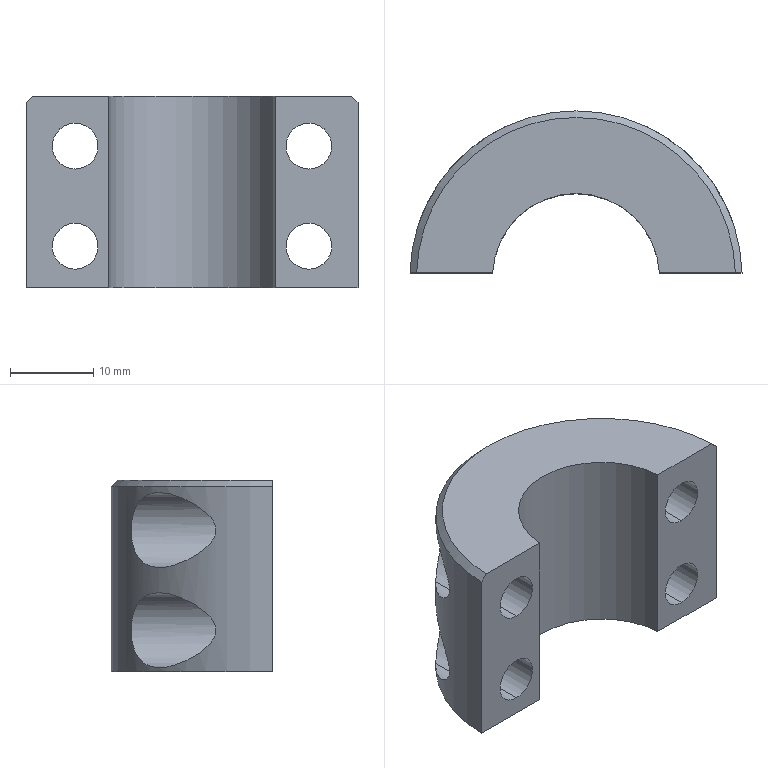Part | STEP file | _GAY12-D20-002.stp | 1 solid | 27 faces | box 39.787 x 19.4 x 23 mm | volume 7951 mm3 | cylinder 18 | plane 8 | cone 1 | commonest cylinder face diameters 5.5 x8 9 x8 20 x1 39.8 x1